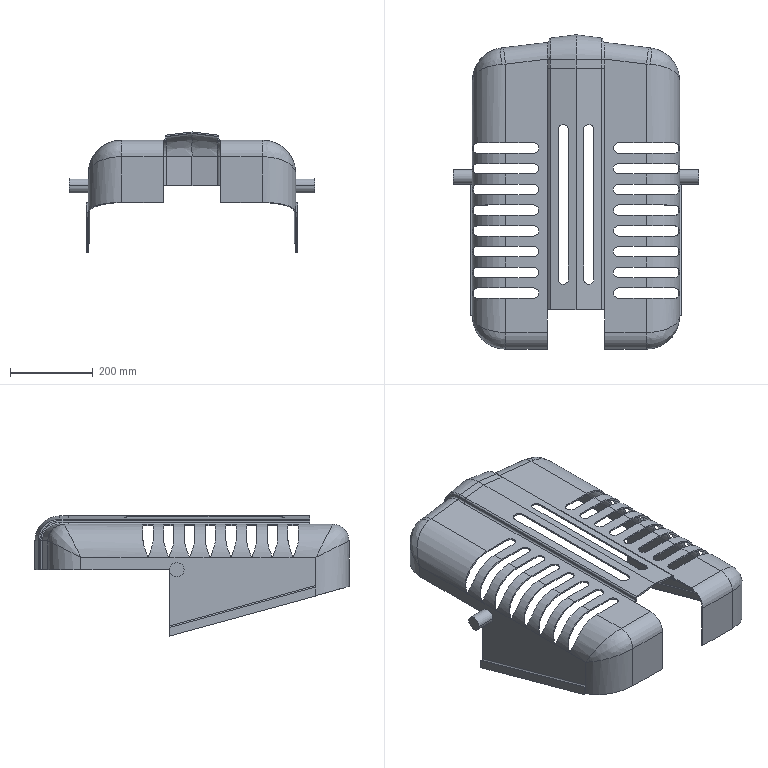Part | SolidWorks | 1 solid | 294 faces | box 593 x 758 x 290 mm | volume 1986947 mm3 | cylinder 148 | plane 122 | spline 24 | commonest cylinder face diameters 25 x60 153 x22 160 x22 8 x14 15 x8 1 x6